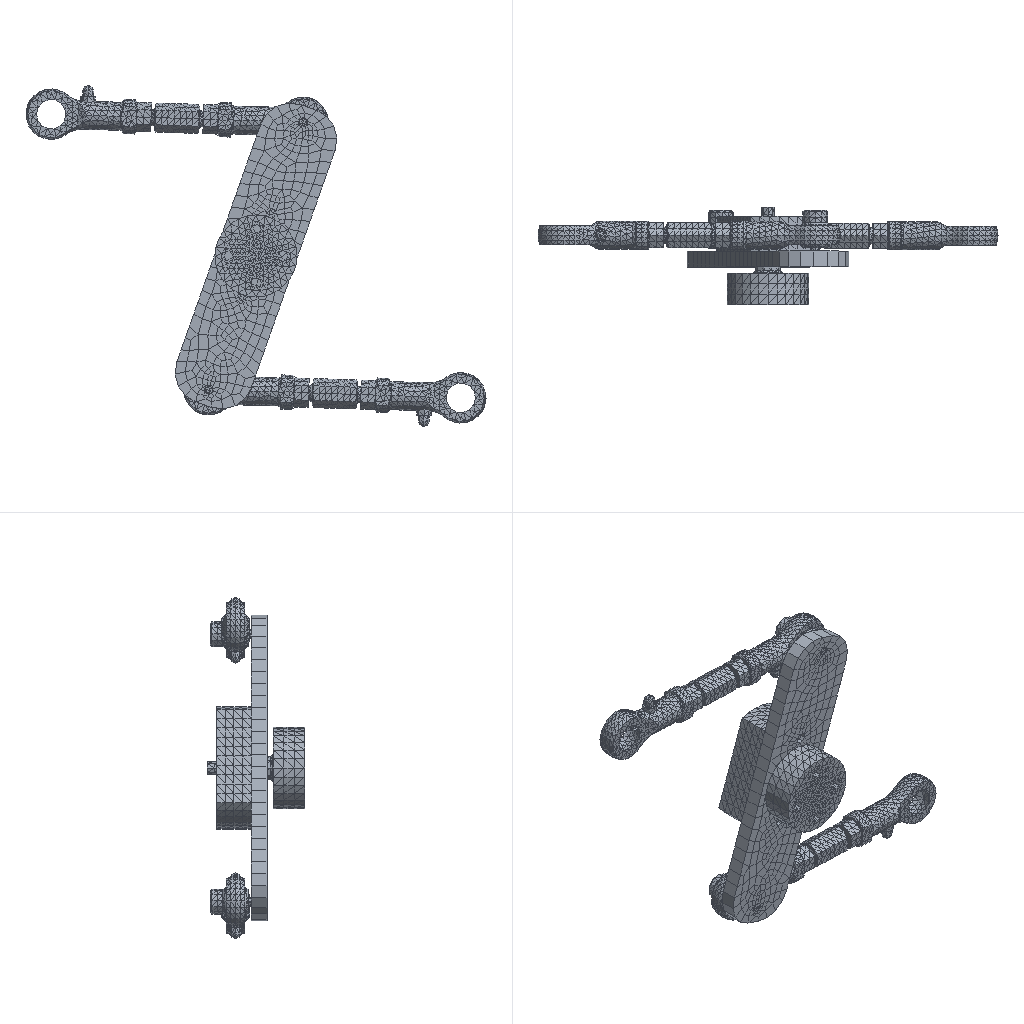Simulation study | abaqus
Set-up summary:
category,name,step,type,value,unit,region
solver,abaqus
solver,version,,,Abaqus/Explicit 2020
units,not stated in the deck,,not stated
analysis,deck,,transient,transient
load_step,Step-1,Step-1,transient
load_step,requested,,,1
mesh,nodes,,,13008
mesh,elements,,,49605
element_type,C3D4,,solid,49230
element_type,C3D8R,,solid,375
load,load commands in deck,,count,2
bc,support commands in deck,,count,18
material,MATERIAL-1,,in results
check,setup vs results,,match,"per instance, exact: element labels, types and connectivity; labels of the nodes the elements use; coordinates not compared"
Abaqus input file, long lists of numbers shortened:
*Heading
** Job name: Job-1 Model name: Model-1
** Generated by: Abaqus/CAE 2020
*Preprint, echo=NO, model=NO, history=NO, contact=NO
**
** PARTS
**
*Part, name=bi1
*Node
      1,   64.873,          22.,   -20.419
      2,   61.874,          22.,  -20.323
** (2411 more lines like these left out)
*Element, type=C3D4
 1, 1495, 1496,  882, 1497
 2, 1495, 1497,  882,    3
** (9696 more lines like these left out)
*Nset, nset=Set-4, generate
    1,  2413,     1
*Elset, elset=Set-4, generate
    1,  9698,     1
** Section: Section-1
*Solid Section, elset=Set-4, material=Material-1
,
*End Part
**
*Part, name=bi2
*Node
      1,   168.561,          22.,  -118.577
      2,   171.56,          22.,  -118.673
** (2419 more lines like these left out)
*Element, type=C3D4
 1, 1498, 1499,  884, 1500
 2, 1498, 1500,  884,    3
** (9732 more lines like these left out)
*Nset, nset=Set-4, generate
    1,  2421,     1
*Elset, elset=Set-4, generate
    1,  9734,     1
** Section: Section-1
*Solid Section, elset=Set-4, material=Material-1
,
*End Part
**
*Part, name=part-12
*End Part
**
*Part, name=part-14
*End Part
**
*Part, name=part-15
*End Part
**
*Part, name=part-16
*End Part
**
*Part, name=part-17
*End Part
**
*Part, name=part-18
*End Part
**
*Part, name=part-21
*End Part
**
*Part, name=part-22
*End Part
**
*Part, name=part-25
*End Part
**
*Part, name=part-26
*End Part
**
**
** ASSEMBLY
**
*Assembly, name=Assembly
**
*Instance, name=part-12-1, part=part-12
*Node
      1,   101.66,   18.3,  -114.431
      2,   101.82,   18.3,  -109.434
** (902 more lines like these left out)
*Element, type=C3D4
   1, 547, 548,   9, 549
   2,  57, 550, 551, 549
** (3698 more lines like these left out)
*Nset, nset=Set-1, generate
   1,  904,    1
*Elset, elset=Set-1, generate
    1,  3700,     1
** Section: Section-1
*Solid Section, elset=Set-1, material=Material-1
,
*End Instance
**
*Instance, name=part-14-1, part=part-14
*Node
      1,   131.774,   18.3,  -24.565
      2,   131.614,   18.3,  -29.562
** (911 more lines like these left out)
*Element, type=C3D4
   1, 398, 547, 548, 549
   2, 397, 549, 547, 398
** (3740 more lines like these left out)
*Nset, nset=Set-1, generate
   1,  913,    1
*Elset, elset=Set-1, generate
    1,  3742,     1
** Section: Section-1
*Solid Section, elset=Set-1, material=Material-1
,
*End Instance
**
*Instance, name=part-15-1, part=part-15
*Node
      1,   125.11,   26.15,  -72.46
      2,   108.324,   26.15,   -66.536
** (1092 more lines like these left out)
*Element, type=C3D4
   1,  739,  740,  741,  742
   2,  739,  740,  742,  743
** (4180 more lines like these left out)
*Nset, nset=Set-1, generate
    1,  1094,     1
*Elset, elset=Set-1, generate
    1,  4182,     1
** Section: Section-1
*Solid Section, elset=Set-1, material=Material-1
,
*End Instance
**
*Instance, name=part-16-1, part=part-16
*Node
      1,    114.514,          25.,  -71.954
      2,    114.714,   24.7,  -71.731
** (2459 more lines like these left out)
*Element, type=C3D4
    1, 1285, 1286, 1287, 1288
    2,  618,  538, 1289,  617
** (10806 more lines like these left out)
*Nset, nset=Set-1, generate
    1,  2461,     1
*Elset, elset=Set-1, generate
     1,  10808,      1
** Section: Section-1
*Solid Section, elset=Set-1, material=Material-1
,
*End Instance
**
*Instance, name=part-17-1, part=part-17
*Node
      1,   131.654,          12.,  -28.563
      2,   131.735,          12.,  -25.564
** (236 more lines like these left out)
*Element, type=C3D4
  1, 174,  14, 167,  97
  2, 174, 175, 158, 167
** (823 more lines like these left out)
*Nset, nset=Set-1, generate
   1,  238,    1
*Elset, elset=Set-1, generate
   1,  825,    1
** Section: Section-1
*Solid Section, elset=Set-1, material=Material-1
,
*End Instance
**
*Instance, name=part-18-1, part=part-18
*Node
      1,   100.865,          12.,  -113.151
      2,   102.614,          12.,  -110.713
** (240 more lines like these left out)
*Element, type=C3D4
  1, 175,  95, 176,  84
  2, 175, 148, 176, 177
** (842 more lines like these left out)
*Nset, nset=Set-1, generate
   1,  242,    1
*Elset, elset=Set-1, generate
   1,  844,    1
** Section: Section-1
*Solid Section, elset=Set-1, material=Material-1
,
*End Instance
**
*Instance, name=part-21-1, part=part-21
*Node
      1,   114.717,          31.,  -69.498
      2,   118.717,          31.,  -69.498
** (1015 more lines like these left out)
*Element, type=C3D4
   1,  617,  245,  173,   39
   2,  618,  619,  620,  621
** (4115 more lines like these left out)
*Nset, nset=Set-1, generate
    1,  1017,     1
*Elset, elset=Set-1, generate
    1,  4117,     1
** Section: Section-1
*Solid Section, elset=Set-1, material=Material-1
,
*End Instance
**
*Instance, name=part-22-1, part=part-22
*Node
      1,   102.433,          17.,   -117.479
      2,   97.718,          17.,  -115.815
** (838 more lines like these left out)
*Element, type=C3D8R
  1, 140,  57,  58, 108, 560, 477, 478, 528
  2, 108, 174,   2, 371, 528, 594, 422, 791
** (373 more lines like these left out)
*Nset, nset=Set-1, generate
   1,  840,    1
*Elset, elset=Set-1, generate
   1,  375,    1
** Section: Section-1
*Solid Section, elset=Set-1, material=Material-1
,
*End Instance
**
*Instance, name=part-25-1, part=part-25
*Node
      1,    121.543,   13.6,    -57.824
      2,    121.543,   13.6,    -53.824
** (231 more lines like these left out)
*Element, type=C3D4
  1, 174,  54, 175, 176
  2, 174, 177,  54,  55
** (789 more lines like these left out)
*Nset, nset=Set-1, generate
   1,  233,    1
*Elset, elset=Set-1, generate
   1,  791,    1
** Section: Section-1
*Solid Section, elset=Set-1, material=Material-1
,
*End Instance
**
*Instance, name=part-26-1, part=part-26
*Node
      1,    111.891,   13.6,  -85.171
      2,    111.891,   13.6,  -81.171
** (230 more lines like these left out)
*Element, type=C3D4
  1, 174, 175,  52, 111
  2, 174,  53, 176, 146
** (787 more lines like these left out)
*Nset, nset=Set-1, generate
   1,  232,    1
*Elset, elset=Set-1, generate
   1,  789,    1
** Section: Section-1
*Solid Section, elset=Set-1, material=Material-1
,
*End Instance
**
*Instance, name=bi1-1, part=bi1
*End Instance
**
*Instance, name=bi2-1, part=bi2
*End Instance
**
*Node
      1,   181.699,          22.,  -114.496
*Node
      2,   51.735,          22.,        -24.5
*Nset, nset=Set-1, instance=part-21-1
  51,  52,  53,  54,  55,  56,  57,  58,  61,  62, 241, 242, 243, 246, 247, 248
 249, 250, 251, 254, 255, 256, 257, 258, 259, 262, 263, 264, 269, 270, 271, 272
** (13 more lines like these left out)
*Elset, elset=Set-1, instance=part-21-1
   72,  152,  362,  393,  399,  419,  430,  501,  588,  599,  650,  730,  742,  758,  767,  824
  894,  929,  939,  953,  964,  967, 1001, 1002, 1003, 1005, 1006, 1007, 1008, 1024, 1025, 1039
** (24 more lines like these left out)
*Nset, nset=Set-13, instance=part-21-1
  45,  46,  51,  52,  53,  54,  55,  56,  57,  58,  61,  62, 203, 204, 205, 206
 207, 208, 209, 210, 211, 212, 213, 214, 215, 216, 217, 218, 219, 220, 221, 222
** (18 more lines like these left out)
*Elset, elset=Set-13, instance=part-21-1
   72,   73,  152,  278,  299,  362,  393,  399,  415,  419,  430,  501,  588,  599,  650,  730
  742,  758,  767,  790,  804,  821,  822,  824,  834,  851,  888,  890,  894,  907,  929,  939
** (34 more lines like these left out)
*Nset, nset=Set-16
 1,
*Nset, nset=Set-17
 2,
*Nset, nset=Set-18, instance=part-21-1
  45,  46,  51,  52,  53,  54,  55,  56,  57,  58,  61,  62, 203, 204, 205, 206
 207, 208, 209, 210, 211, 212, 213, 214, 215, 216, 217, 218, 219, 220, 221, 222
** (18 more lines like these left out)
*Elset, elset=Set-18, instance=part-21-1
   72,   73,  152,  278,  299,  362,  393,  399,  415,  419,  430,  501,  588,  599,  650,  730
  742,  758,  767,  790,  804,  821,  822,  824,  834,  851,  888,  890,  894,  907,  929,  939
** (34 more lines like these left out)
*Nset, nset=Set-19, instance=part-12-1
   5,   6,   9,  10,  63,  64,  65,  66,  67,  68,  69,  70,  71,  72,  73,  74
  75,  76,  77,  78,  97,  98,  99, 100, 101, 102, 103, 104, 105, 106, 107, 108
** (1 more lines like these left out)
*Nset, nset=Set-19, instance=part-15-1
  11,  12,  15,  16,  21,  22,  23,  24,  25,  26, 235, 236, 237, 238, 239, 240
 241, 242, 243, 244, 245, 246, 247, 248, 249, 250, 251, 252, 253, 254, 255, 256
** (11 more lines like these left out)
*Nset, nset=Set-19, instance=part-16-1
   9,  10,  13,  14, 123, 124, 125, 126, 127, 128, 129, 130, 131, 132, 133, 134
 135, 136, 137, 138, 139, 140, 141, 142, 143, 144, 145, 146, 147, 148, 169, 170
** (11 more lines like these left out)
*Nset, nset=Set-19, instance=part-26-1
   9,  10,  11,  12,  13,  14,  15,  16,  82,  83,  84,  85,  86,  87,  88,  89
  90,  91,  92,  93,  94,  95,  96,  97,  98,  99, 159, 160, 161, 162
*Nset, nset=Set-19, instance=part-17-1
  13,  14,  15,  16,  17,  18,  19,  20,  92,  93,  94,  95,  96,  97,  98,  99
 100, 101, 102, 103, 104, 105, 106, 107, 157, 158, 159, 160, 161, 162, 163, 164
** (1 more lines like these left out)
*Nset, nset=Set-19, instance=part-21-1
   1,   2,  63,  64,  65,  66,  67,  68, 309, 310, 311
*Nset, nset=Set-19, instance=part-25-1
   9,  10,  11,  12,  13,  14,  15,  16,  82,  83,  84,  85,  86,  87,  88,  89
  90,  91,  92,  93,  94,  95,  96,  97,  98,  99, 159, 160, 161, 162
*Nset, nset=Set-19, instance=bi1-1
  173,  174,  176,  177,  179,  181,  183,  192,  193,  723,  724,  725,  726,  727,  728,  730
  731,  732,  733,  734,  735,  739,  740,  741,  742,  743,  760,  761,  762,  763,  764,  765
** (2 more lines like these left out)
*Nset, nset=Set-19, instance=bi2-1
  173,  174,  176,  177,  179,  181,  183,  192,  193,  723,  724,  725,  726,  727,  728,  730
  731,  732,  733,  734,  735,  739,  740,  741,  742,  743,  760,  761,  762,  763,  764,  765
** (2 more lines like these left out)
*Elset, elset=Set-19, instance=part-12-1
  529, 1391, 1544, 1580, 1793, 1896, 1922, 2045, 2095, 2105, 2297, 2300, 2389, 2485, 2554, 2574
 2587, 2631, 2651, 2654, 2675, 2757, 2931, 2982, 3003, 3010, 3015, 3048, 3052, 3062, 3067, 3085
** (1 more lines like these left out)
*Elset, elset=Set-19, instance=part-15-1
   39,   98,  111,  115,  204,  266,  284,  366,  388,  405,  438,  501,  524,  542,  550,  595
  626,  695,  734,  749,  755,  830,  932,  947,  981,  986,  992, 1005, 1031, 1060, 1100, 1133
** (17 more lines like these left out)
*Elset, elset=Set-19, instance=part-16-1
   115,   291,   394,   492,   829,  1144,  1250,  1633,  1661,  1672,  1695,  1741,  1766,  1779,  1788,  1797
  1803,  1814,  1849,  1852,  1862,  1863,  1866,  2004,  2074,  2107,  2184,  2214,  2383,  2481,  2524,  2539
** (18 more lines like these left out)
*Elset, elset=Set-19, instance=part-26-1
  21,  53,  56, 145, 186, 217, 220, 227, 230, 264, 269, 482, 500, 505, 508, 512
 513, 515, 518, 521, 531, 537, 540, 546, 555, 558, 564, 565, 573, 607, 611, 614
** (1 more lines like these left out)
*Elset, elset=Set-19, instance=part-17-1
   1,  76, 133, 135, 142, 152, 168, 226, 229, 254, 284, 309, 388, 421, 428, 446
 449, 483, 485, 505, 513, 515, 516, 526, 527, 528, 531, 533, 537, 539, 550, 556
** (1 more lines like these left out)
*Elset, elset=Set-19, instance=part-21-1
  431,  455, 1127, 1699, 1786, 1798, 1800, 1823, 1854, 1860, 1878, 1894
*Elset, elset=Set-19, instance=part-25-1
  16,  19,  65, 136, 165, 170, 267, 276, 372, 470, 485, 493, 500, 503, 504, 506
 517, 518, 520, 521, 525, 532, 535, 540, 566, 573, 575, 580, 607, 620, 622, 627
** (1 more lines like these left out)
*Elset, elset=Set-19, instance=bi1-1
  690,  696,  697, 1938, 2433, 2476, 2477, 2531, 2599, 2663, 2839, 2840, 2907, 3026, 3120, 3207
 3343, 3589, 3598, 3612, 3620, 3667, 3815, 4898, 5199, 5350, 5898, 5905, 7300, 7438, 7637, 7686
** (3 more lines like these left out)
*Elset, elset=Set-19, instance=bi2-1
 1908, 2038, 2531, 2688, 2689, 2745, 3155, 3198, 3248, 3278, 3394, 3438, 3439, 3582, 3717, 3866
 3907, 3928, 3971, 4243, 4299, 4300, 4441, 4515, 4728, 4923, 4926, 5077, 5764, 6008, 6688, 6708
** (3 more lines like these left out)
*Nset, nset=m_Set-14
 1,
*Nset, nset=m_Set-15
 2,
*Elset, elset=_m_Surf-1_S1, internal, instance=part-22-1, generate
   1,  375,    1
*Surface, type=ELEMENT, name=m_Surf-1
_m_Surf-1_S1, S1
*Elset, elset=_m_Surf-5_S3, internal, instance=part-17-1
  96,  98, 131, 172, 188, 209, 231, 235, 236, 239, 240, 241, 281, 308, 327, 496
 497, 545, 547, 557, 561, 564, 617, 631, 647, 692, 733, 784, 785, 787, 795, 796
** (1 more lines like these left out)
*Elset, elset=_m_Surf-5_S1, internal, instance=part-17-1
 97,
*Surface, type=ELEMENT, name=m_Surf-5
_m_Surf-5_S3, S3
_m_Surf-5_S1, S1
*Elset, elset=_m_Surf-7_S3, internal, instance=part-18-1
 192, 196, 256, 267, 268, 270, 271, 278, 349, 351, 352, 567, 568, 611, 632, 686
 719, 727, 730, 746, 787, 793, 794, 795, 796, 798, 800, 801, 803, 806, 807, 809
** (1 more lines like these left out)
*Elset, elset=_m_Surf-7_S2, internal, instance=part-18-1
 311,
*Elset, elset=_m_Surf-7_S1, internal, instance=part-18-1
 394, 811
*Surface, type=ELEMENT, name=m_Surf-7
_m_Surf-7_S3, S3
_m_Surf-7_S2, S2
_m_Surf-7_S1, S1
*Elset, elset=_s_Surf-1_S3, internal, instance=part-15-1
  109,  125,  129,  173,  175,  352,  398,  431,  519,  552,  569,  663,  664,  665,  705,  707
  732,  748,  863,  868,  952, 1167, 1364, 1423, 1534, 1591, 1593, 1594, 1596, 1637, 1645, 1647
** (7 more lines like these left out)
*Elset, elset=_s_Surf-1_S2, internal, instance=part-15-1
  440, 1057, 1363, 1620, 1861, 2056, 2103, 2225, 2312, 2896, 2920, 2922, 2939, 2994, 3043, 3068
 3080, 3084, 3172, 3179, 3187, 3199, 3234, 3252, 3292, 3318, 3340, 3360, 3400, 3407, 3489, 3542
** (1 more lines like these left out)
*Elset, elset=_s_Surf-1_S4, internal, instance=part-15-1
 1112, 1361, 1481, 1753, 2126, 2232, 2234, 2400, 2410, 2803, 2956, 3079, 3110, 3139, 3170, 3198
 3200, 3254, 3294, 3319, 3327, 3334, 3519, 3555, 3581, 3588, 3607, 3729, 3883, 3918, 3927, 3970
** (1 more lines like these left out)
*Elset, elset=_s_Surf-1_S1, internal, instance=part-15-1
 1228, 1562, 1734, 2116, 2832, 2926, 3099, 3112, 3117, 3264, 3295, 3563, 3594, 3596, 3648, 3911
 3913, 3982, 4033, 4052, 4086
*Surface, type=ELEMENT, name=s_Surf-1
_s_Surf-1_S3, S3
_s_Surf-1_S2, S2
_s_Surf-1_S4, S4
_s_Surf-1_S1, S1
*Elset, elset=_s_Surf-3_S3, internal, instance=bi2-1
 1745, 1760, 1803, 1813, 1934, 1938, 1939, 2113, 2169, 2268, 2437, 2488, 2535, 2601, 2628, 2648
 2656, 2661, 2665, 2676, 2677, 2693, 2704, 2705, 2708, 2711, 2740, 2741, 2743, 2744, 2747, 2762
** (7 more lines like these left out)
*Elset, elset=_s_Surf-3_S4, internal, instance=bi2-1
  445, 3759, 4487, 5479, 6660, 9379
*Elset, elset=_s_Surf-3_S2, internal, instance=bi2-1
 1732, 2886, 2888
*Elset, elset=_s_Surf-3_S1, internal, instance=bi2-1
 2573, 5276, 6246, 6672, 7266, 7420
*Surface, type=ELEMENT, name=s_Surf-3
_s_Surf-3_S3, S3
_s_Surf-3_S4, S4
_s_Surf-3_S2, S2
_s_Surf-3_S1, S1
*Elset, elset=_s_Surf-4_S3, internal, instance=bi1-1
 1803, 1817, 1830, 1847, 1955, 2185, 2237, 2293, 2307, 2333, 2416, 2450, 2503, 2512, 2542, 2616
 2658, 2666, 2667, 2686, 2687, 2699, 2715, 2718, 2730, 2743, 2749, 2757, 2766, 2767, 2771, 2775
** (7 more lines like these left out)
*Elset, elset=_s_Surf-4_S4, internal, instance=bi1-1
 2548, 2697, 2707, 2874, 2910, 3201, 3247, 6183
*Elset, elset=_s_Surf-4_S2, internal, instance=bi1-1
 2879, 2884, 2962, 3135, 3281
*Elset, elset=_s_Surf-4_S1, internal, instance=bi1-1
 4896, 5172, 5180, 6181
*Surface, type=ELEMENT, name=s_Surf-4
_s_Surf-4_S3, S3
_s_Surf-4_S4, S4
_s_Surf-4_S2, S2
_s_Surf-4_S1, S1
*Elset, elset=_s_Surf-5_S3, internal, instance=part-22-1
 28,
*Elset, elset=_s_Surf-5_S6, internal, instance=part-22-1
 30, 32, 93
*Elset, elset=_s_Surf-5_S4, internal, instance=part-22-1
 23, 49, 82, 83
*Surface, type=ELEMENT, name=s_Surf-5
_s_Surf-5_S3, S3
_s_Surf-5_S6, S6
_s_Surf-5_S4, S4
*Elset, elset=_s_Surf-7_S4, internal, instance=part-22-1
  1, 39, 54, 86, 87
*Elset, elset=_s_Surf-7_S5, internal, instance=part-22-1
 84,
*Elset, elset=_s_Surf-7_S6, internal, instance=part-22-1
 38, 89
*Surface, type=ELEMENT, name=s_Surf-7
_s_Surf-7_S4, S4
_s_Surf-7_S5, S5
_s_Surf-7_S6, S6
** Constraint: Constraint-1
*Tie, name=Constraint-1, adjust=yes
s_Surf-1, m_Surf-1
** Constraint: Constraint-2
*Coupling, constraint name=Constraint-2, ref node=m_Set-14, surface=s_Surf-3
*Kinematic
** Constraint: Constraint-3
*Coupling, constraint name=Constraint-3, ref node=m_Set-15, surface=s_Surf-4
*Kinematic
*End Assembly
*Amplitude, name=Amp-1
             0.,              0.,           0.001,              1.
**
** MATERIALS
**
*Material, name=Material-1
*Density
 7.8e-09,
*Elastic
210000., 0.25
**
** INTERACTION PROPERTIES
**
*Surface Interaction, name=IntProp-1
*Friction
 0.1,
*Surface Behavior, pressure-overclosure=HARD
**
** BOUNDARY CONDITIONS
**
** Name: BC-4 Type: 位移/转角
*Boundary
Set-18, 1, 1
Set-18, 2, 2
Set-18, 3, 3
Set-18, 4, 4
Set-18, 6, 6
**
** INTERACTIONS
**
** Interaction: Int-1
*Contact, op=NEW
*Contact Inclusions, ALL EXTERIOR
*Contact Property Assignment
 ,  , IntProp-1
** ----------------------------------------------------------------
**
** STEP: Step-1
**
*Step, name=Step-1, nlgeom=YES
*Dynamic, Explicit
, 0.001
*Bulk Viscosity
0.06, 1.2
**
** BOUNDARY CONDITIONS
**
** Name: BC-2 Type: 位移/转角
*Boundary, amplitude=Amp-1
Set-16, 1, 1, 13.5
Set-16, 2, 2
Set-16, 3, 3
Set-16, 4, 4
Set-16, 5, 5
Set-16, 6, 6
** Name: BC-3 Type: 位移/转角
*Boundary, amplitude=Amp-1
Set-17, 1, 1, -13.5
Set-17, 2, 2
Set-17, 3, 3
Set-17, 4, 4
Set-17, 5, 5
Set-17, 6, 6
** Name: BC-5 Type: 位移/转角
*Boundary
Set-19, 2, 2
**
** OUTPUT REQUESTS
**
*Restart, write, number interval=1, time marks=NO
**
** FIELD OUTPUT: F-Output-1
**
*Output, field, variable=PRESELECT
**
** HISTORY OUTPUT: H-Output-1
**
*Output, history
*Node Output, nset=m_Set-14
RF1, RM
**
** HISTORY OUTPUT: H-Output-2
**
*Node Output, nset=m_Set-15
RF1, RM
*End Step
Results summary:
result,step,Step-1,completed,increments=70055 time=0.001/0.001
result,analysis,,,transient
result,last_loadstep,,,1
result,primary field,,,U
result,reaction total,,FX,6651.395,model units
result,reaction total,,FY,1498.338,model units
result,reaction total,,FZ,507.497,model units